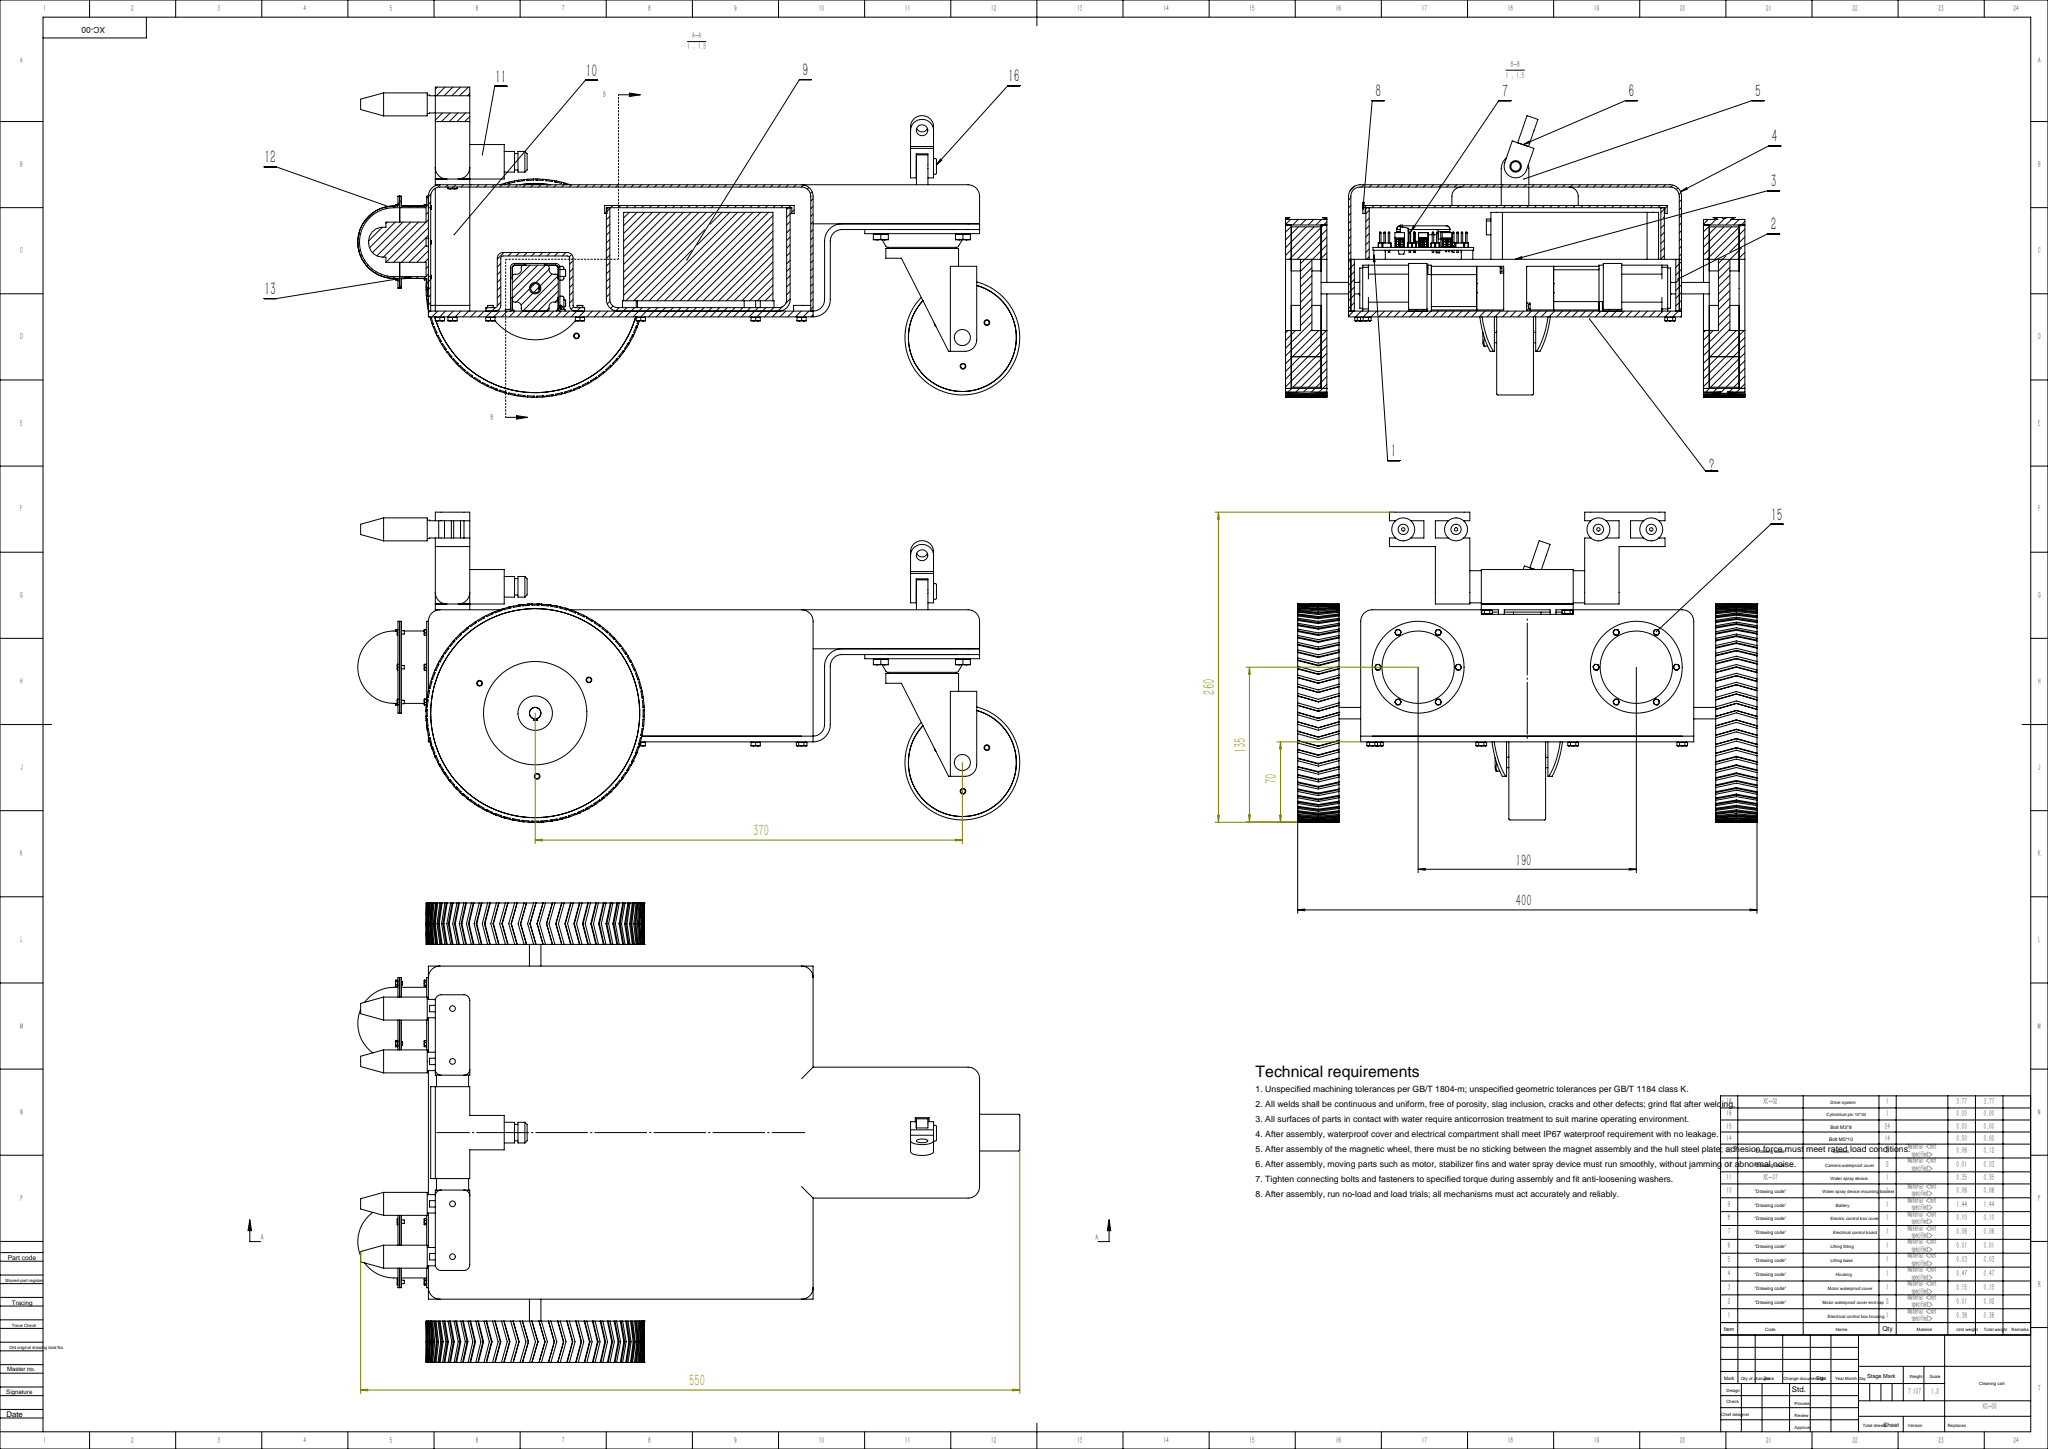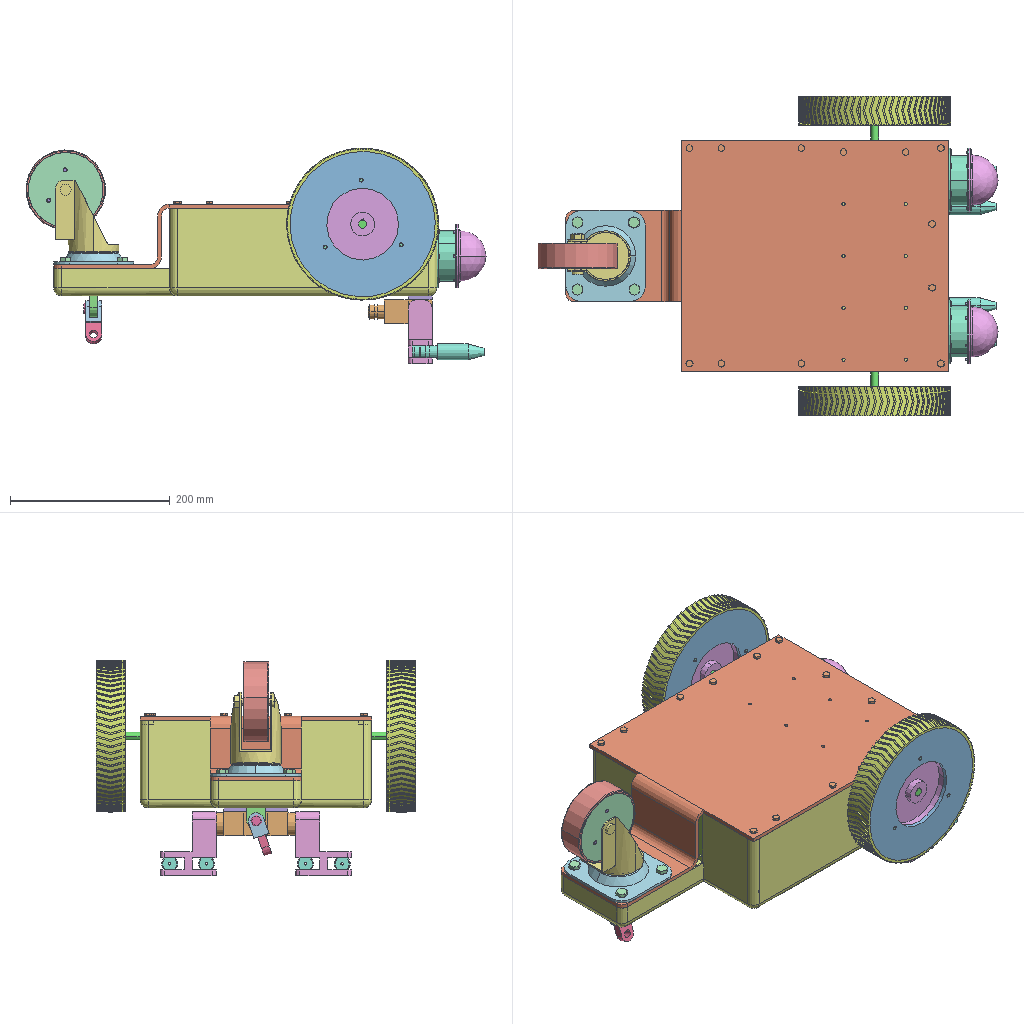Assembly | SolidWorks | 42 different items | 115 placed | box 576 x 400 x 270 mm
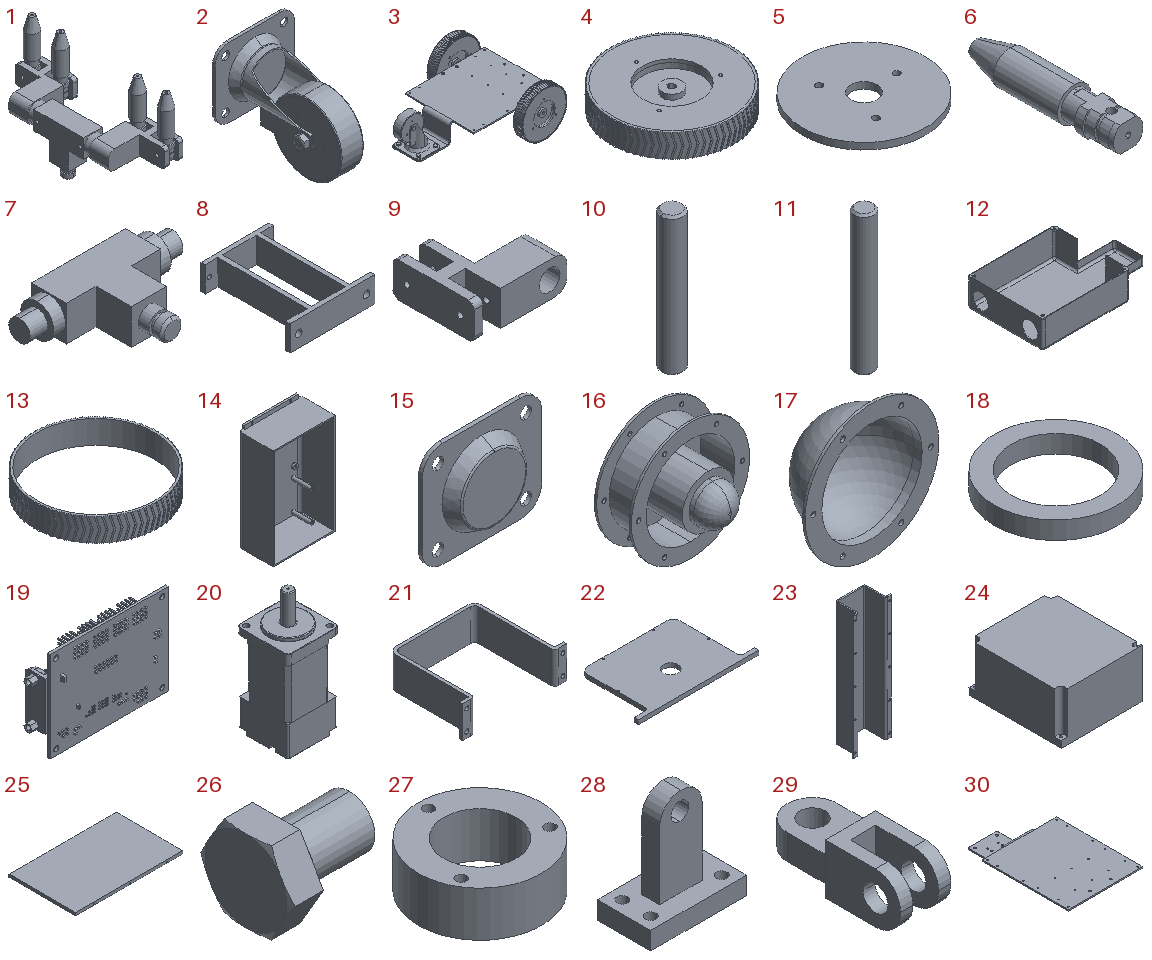Parts list (item | name | quantity | parent item | size | volume | features):
1 | (subassembly) | x1 | - | 80 x 240 x 145 mm | 354979 mm3 | -
2 | (subassembly) | x1 | in 3 | 114 x 144 x 135 mm | 347724 mm3 | features CompositeCurve 1
3 | (subassembly) | x1 | - | 517.127 x 400 x 190.253 mm | 2987569 mm3 | features CompositeCurve 2, LocalLPattern 1
4 | (subassembly) | x2 | in 3 | 190.182 x 190.182 x 36 mm | 833820 mm3 | -
5 | - | x2 | in 2 | 94 x 94 x 5 mm | 32834 mm3 | features Extrusion 1
6 | - | x4 | in 1 | 20 x 90 x 20 mm | 21802 mm3 | features ICE 3, Revolution 1
7 | - | x1 | in 1 | 130 x 80 x 30 mm | 123416 mm3 | features ICE 6, Chamfer 1, Cut 1, Extrusion 1
8 | - | x1 | - | 100 x 115 x 30 mm | 57801 mm3 | features ICE 2, Extrusion 1
9 | - | x2 | in 1 | 80 x 70 x 30 mm | 72177 mm3 | features ICE 3, Fillet 2, Extrusion 1
10 | - | x3 | in 2 | 5 x 5 x 32 mm | 624.653 mm3 | features Chamfer 1, Extrusion 1
11 | - | x6 | in 4 | 5 x 5 x 36 mm | 703.193 mm3 | features Chamfer 1, Extrusion 1
12 | - | x1 | - | 480 x 290 x 110 mm | 467348 mm3 | features ICE 6, Fillet 3, CirPattern 2, Extrusion 1, Shell 1
13 | - | x2 | in 4 | 190.182 x 190.182 x 36 mm | 68309 mm3 | features CirPattern 1, Extrusion 1, ICE 1
14 | - | x1 | - | 160 x 90 x 280 mm | 364305 mm3 | features ICE 5, Extrusion 1, Fillet 1, Shell 1
15 | - | x1 | in 2 | 114 x 15.475 x 100 mm | 79826 mm3 | features RefAxis 6, 3DProfileFeature 2, ICE 2, Extrusion 1, Revolution 1
16 | - | x2 | - | 80 x 52 x 80 mm | 58059 mm3 | features ICE 5, Fillet 1, Revolution 1
17 | - | x2 | - | 80 x 36.5 x 80 mm | 13163 mm3 | features ICE 1, Revolution 1
18 | - | x2 | in 4 | 180 x 180 x 26 mm | 316515 mm3 | features Extrusion 1
19 | - | x1 | - | - | 58876 mm3 | features BaseBody 155, Scale 1
20 | - | x2 | in 3 | 40 x 46.5 x 96 mm | 102158 mm3 | features BaseBody 5
21 | - | x2 | in 3 | 52 x 41.5 x 16 mm | 3067 mm3 | features Extrusion 1, ICE 1
22 | - | x2 | - | 86 x 51 x 3 mm | 9982 mm3 | features Extrusion 1
23 | - | x1 | - | 86 x 51 x 280 mm | 147456 mm3 | features Extrusion 1, ICE 1, LPattern 1
24 | - | x1 | - | 130 x 150 x 77 mm | 1439024 mm3 | features ICE 2, Extrusion 1
25 | - | x1 | - | 265 x 165 x 7 mm | 95885 mm3 | features ICE 2, Extrusion 1, LPattern 1
26 | - | x24 | - | 6.1 x 5.543 x 4.8 mm | 68.566 mm3 | features RevCut 3, Boss 1, Chamfer 1, Extrusion 1, Fillet 1, ICE 1, LPattern 1, Scale 1
27 | - | x1 | in 2 | 60 x 60 x 22 mm | 39741 mm3 | features Extrusion 1
28 | - | x1 | - | 54 x 30 x 60 mm | 25666 mm3 | features ICE 2, Extrusion 1, Fillet 1
29 | - | x1 | - | 20 x 55 x 20 mm | 9495 mm3 | features ICE 2, Extrusion 1
30 | - | x1 | in 3 | 290 x 480 x 81 mm | 601902 mm3 | features Cut 5, ICE 4, Fillet 3, Extrusion 1
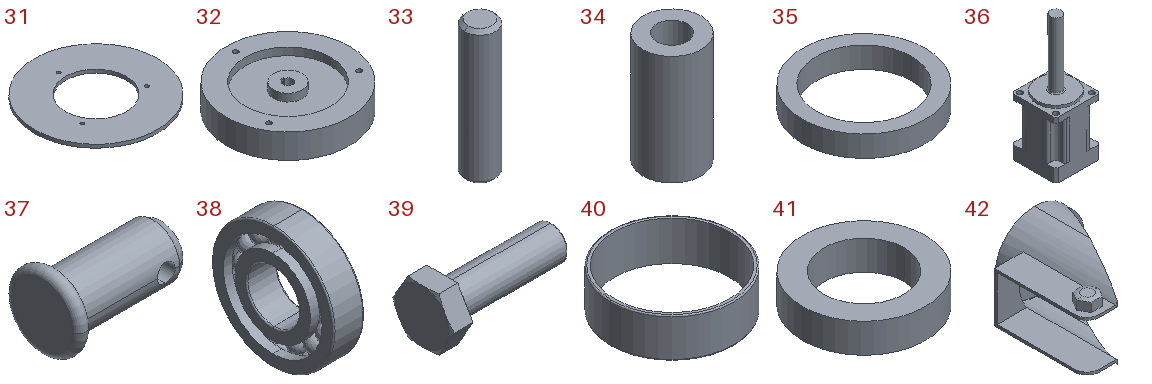31 | - | x4 | in 4 | 182 x 182 x 5 mm | 97974 mm3 | features Extrusion 1
32 | - | x2 | in 4 | 130 x 130 x 26 mm | 250937 mm3 | features ICE 3, Extrusion 1
33 | - | x1 | in 2 | 9 x 9 x 39 mm | 2455 mm3 | features Chamfer 1, Extrusion 1
34 | - | x1 | in 2 | 17 x 17 x 32 mm | 5228 mm3 | features Extrusion 1
35 | - | x1 | in 2 | 35 x 35 x 6 mm | 2337 mm3 | features Extrusion 1
36 | - | x2 | in 3 | 40 x 40 x 114 mm | 76239 mm3 | features ICE 5, BaseBody 1
37 | - | x1 | - | 22.5 x 14 x 14 mm | 1821 mm3 | features Cut 1, Fillet 1, Revolution 1
38 | - | x2 | in 2 | 7 x 28 x 28 mm | 2641 mm3 | features Revolution 3, CirPattern 1, Fillet 1
39 | - | x25 | in 3 | 19.5 x 9.238 x 8 mm | 500.222 mm3 | features RevCut 3, Boss 1, Chamfer 1, Extrusion 1, Fillet 1, LPattern 1
40 | - | x1 | in 2 | 100 x 100 x 32 mm | 29120 mm3 | features Extrusion 1, Fillet 1
41 | - | x1 | in 2 | 92 x 92 x 22 mm | 84044 mm3 | features Extrusion 1
42 | - | x1 | in 2 | 79.167 x 90.525 x 63.333 mm | 28539 mm3 | features RefAxis 15, ICE 6, 3DProfileFeature 5, Revolution 2
Mates (type | each side: item.copy, entity, surface, feature):
In the top assembly
Coincident | 23.1 face plane Boss-Extrude1 | 22.1 face plane Boss-Extrude1 | 3 times
Coincident | 23.1 face plane Boss-Extrude1 | 22.2 face plane Boss-Extrude1
Coincident | 7.1 face plane Boss-Extrude1 | 8.1 face plane Boss-Extrude1 | 3 times
Concentric | 28.1 face cylinder Cut-Extrude1 | 29.1 face cylinder Boss-Extrude2
Coincident | 28.1 face plane Boss-Extrude2 | 29.1 face plane Cut-Extrude1
DistanceDim | 19.1 face plane Input12 | 14.1 face plane Shell1
Concentric | 14.1 face cylinder Boss-Extrude2 | 19.1 face cylinder Input12
Parallel | 14.1 face plane Shell1 | 19.1 face plane Input12
Concentric | 14.1 face cylinder Boss-Extrude3 | 24.1 face cylinder Boss-Extrude1 | 2 times
Coincident | 14.1 face plane Boss-Extrude3 | 24.1 face plane Boss-Extrude1
Coincident | 14.1 face plane Boss-Extrude1 | 25.1 face plane Boss-Extrude1
DistanceDim | 25.1 face plane Boss-Extrude2 | 14.1 face plane Boss-Extrude1 | 2 times
Concentric | 12.1 face cylinder Cut-Extrude5 | 17.1 face cylinder Revolve1
Concentric | 12.1 face cylinder Cut-Extrude5 | 17.2 face cylinder Revolve1
Coincident | 16.1 face plane Revolve1 | 17.2 face plane Revolve1
Concentric | 12.1 face cylinder Cut-Extrude5 | 16.1 face cylinder Revolve1
Concentric | 12.1 face cylinder Cut-Extrude5 | 16.2 face cylinder Revolve1
Concentric | 12.1 face cylinder Cut-Extrude5 | 16.2 face cylinder Cut-Extrude1
Coincident | 12.1 face plane Boss-Extrude1 | 16.2 face plane Revolve1
Coincident | 17.1 face plane Revolve1 | 16.2 face plane Revolve1
Coincident | 17.2 edge | 16.1 face cylinder Cut-Extrude1
Concentric | 17.1 face cylinder Cut-Extrude1 | 16.2 face cylinder Cut-Extrude1
Concentric | 12.1 face cylinder CirPattern2 | 16.1 face cylinder Cut-Extrude1
Concentric | 8.1 face cylinder Cut-Extrude2 | 39.1 face cylinder BaseBody
Coincident | 8.1 face plane Boss-Extrude1 | 39.1 face plane BaseHead
Concentric | 8.1 face cylinder Cut-Extrude2 | 39.2 face cylinder BaseBody
Coincident | 8.1 face plane Boss-Extrude1 | 39.2 face plane BaseHead
Concentric | 14.1 face cylinder Cut-Extrude1 | 39.3 face cylinder BaseBody
Concentric | 16.1 face cylinder Cut-Extrude1 | 26.1 face cylinder BaseBody
Coincident | 17.2 face plane Revolve1 | 26.1 face plane BaseHead
Concentric | 16.1 face cylinder Cut-Extrude1 | 26.2 face cylinder BaseBody
Coincident | 16.1 face plane Revolve1 | 26.2 face plane BaseHead
Concentric | 16.2 face cylinder Cut-Extrude1 | 26.3 face cylinder BaseBody
Coincident | 16.2 face plane Revolve1 | 26.3 face plane BaseHead
Concentric | 16.2 face cylinder Cut-Extrude1 | 26.4 face cylinder BaseBody
Coincident | 16.2 face plane Revolve1 | 26.4 face plane BaseHead
Concentric | 28.1 face cylinder Boss-Extrude1 | 39.4 face cylinder BaseBody
Coincident | 28.1 face plane Boss-Extrude1 | 39.4 face plane BaseHead
Concentric | 28.1 face cylinder Boss-Extrude1 | 39.5 face cylinder BaseBody
Coincident | 28.1 face plane Boss-Extrude1 | 39.5 face plane BaseHead
Concentric | 28.1 face cylinder Boss-Extrude1 | 39.6 face cylinder BaseBody
Coincident | 28.1 face plane Boss-Extrude1 | 39.6 face plane BaseHead
Concentric | 28.1 face cylinder Boss-Extrude1 | 39.7 face cylinder BaseBody
Coincident | 28.1 face plane Boss-Extrude1 | 39.7 face plane BaseHead
Concentric | 29.1 face cylinder Boss-Extrude2 | 37.1 face cylinder BaseBody
Coincident | 29.1 face plane Boss-Extrude2 | 37.1 edge
Coincident | 12.1 face plane Boss-Extrude1 | 30.1 face plane Boss-Extrude1 | 3 times
In subassembly 3
Concentric | 36.1 face cylinder Cut-Extrude2 | 20.1 face cylinder Motor - Copy-1-1-solid1
Coincident | 36.1 face plane Input1 | 20.1 face plane Motor - Copy-1-1-solid2 | 2 times
Concentric | 36.2 face cylinder Cut-Extrude2 | 20.2 face cylinder Motor - Copy-1-1-solid1
Coincident | 36.2 face plane Input1 | 20.2 face plane Motor - Copy-1-1-solid2 | 2 times
Coincident | 20.1 face plane Motor-1-1-solid1 | 20.2 face plane Motor-1-1-solid1
Coincident | 36.1 face plane Input1 | 30.2 face plane Boss-Extrude1
Coincident | 36.1 face plane Input1 | 21.1 face plane Boss-Extrude1 | 3 times
Concentric | 36.1 face cylinder Input1 | 36.2 face cylinder Input1
DistanceDim | 20.1 face plane Motor-1-1-solid1 | 20.2 face plane Motor-1-1-solid1
Coincident | 36.1 face plane Boss-Extrude1 | 32.1 face plane Boss-Extrude1
Coincident | 36.2 face plane Boss-Extrude1 | 32.2 face plane Boss-Extrude1
Coincident | 36.2 face plane Input1 | 21.2 face plane Boss-Extrude1 | 2 times
Coincident | 21.1 face plane Boss-Extrude1 | 21.2 face plane Boss-Extrude1
Concentric | 36.1 face cylinder Input1 | 32.1 face cylinder Cut-Extrude1
Concentric | 36.2 face cylinder Input1 | 31.1 edge
Coincident | 15.1 face plane Boss-Extrude1 | 30.2 face plane Boss-Extrude3 | 2 times
Coincident | 15.1 face plane Boss-Extrude1 | 30.2 face plane Boss-Extrude2
Concentric | 30.2 face cylinder Cut-Extrude6 | 39.8 face cylinder BaseBody
Coincident | 30.2 face plane Boss-Extrude1 | 39.8 face plane BaseHead
Concentric | 15.1 face cylinder Cut-Extrude2 | 39.9 face cylinder BaseBody
Coincident | 15.1 face plane Boss-Extrude1 | 39.9 face plane BaseHead
Concentric | 15.1 face cylinder Cut-Extrude2 | 39.10 face cylinder BaseBody
Coincident | 15.1 face plane Boss-Extrude1 | 39.10 face plane BaseHead
Concentric | 30.2 face cylinder Cut-Extrude2 | 39.11 face cylinder BaseBody
Coincident | 15.1 face plane Boss-Extrude1 | 39.11 face plane BaseHead
Concentric | 30.2 face cylinder Cut-Extrude7 | 39.12 face cylinder BaseBody
Coincident | 30.2 face plane Boss-Extrude1 | 39.12 face plane BaseHead
Concentric | 30.2 face cylinder Cut-Extrude3 | 39.13 face cylinder BaseBody
Coincident | 30.2 face plane Boss-Extrude1 | 39.13 face plane BaseHead
Coincident | 30.2 edge | 39.14 face cylinder BaseBody
Coincident | 15.1 face plane Boss-Extrude1 | 39.14 face plane BaseHead
In subassembly 4
Concentric | 18.1 face cylinder Boss-Extrude1 | 31.2 face cylinder Boss-Extrude1
Coincident | 18.1 face plane Boss-Extrude1 | 31.2 face plane Boss-Extrude1
Concentric | 18.1 face cylinder Boss-Extrude1 | 31.3 face cylinder Boss-Extrude1
Coincident | 18.1 face plane Boss-Extrude1 | 31.3 face plane Boss-Extrude1
Concentric | 31.2 face cylinder Boss-Extrude1 | 13.1 face cylinder Boss-Extrude1
Coincident | 31.2 face plane Boss-Extrude1 | 13.1 face plane Boss-Extrude1
Concentric | 31.2 face cylinder Boss-Extrude1 | 32.3 face cylinder Boss-Extrude1 | 2 times
Coincident | 18.1 face plane Boss-Extrude1 | 32.3 face plane Boss-Extrude1
Concentric | 31.3 face cylinder Boss-Extrude1 | 32.3 face cylinder Boss-Extrude1
Parallel | 32.3 face plane Cut-Extrude1 | 4.1 plane
Concentric | 31.3 face cylinder Boss-Extrude1 | 11.1 face cylinder Boss-Extrude1
Coincident | 31.3 face plane Boss-Extrude1 | 11.1 face plane Boss-Extrude1
Concentric | 31.3 face cylinder Boss-Extrude1 | 11.2 face cylinder Boss-Extrude1
Coincident | 31.3 face plane Boss-Extrude1 | 11.2 face plane Boss-Extrude1
Concentric | 31.3 face cylinder Boss-Extrude1 | 11.3 face cylinder Boss-Extrude1
Coincident | 31.3 face plane Boss-Extrude1 | 11.3 face plane Boss-Extrude1
In subassembly 2
Coincident | 15.2 plane | 42.1 plane
Coincident | 15.2 axis | 42.1 axis
Concentric | 42.1 face cylinder Boss-Extrude2 | 41.1 face cylinder Boss-Extrude1
Concentric | 41.1 face cylinder Boss-Extrude1 | 5.1 face cylinder Boss-Extrude1
Concentric | 41.1 face cylinder Boss-Extrude1 | 5.2 face cylinder Boss-Extrude1
Coincident | 41.1 face plane Boss-Extrude1 | 5.2 face plane Boss-Extrude1
Coincident | 41.1 face plane Boss-Extrude1 | 5.1 face plane Boss-Extrude1
DistanceDim | 5.2 face plane Boss-Extrude1 | 42.1 face plane Cut-Extrude1
Concentric | 5.1 face cylinder Boss-Extrude1 | 40.1 face cylinder Boss-Extrude1
Coincident | 5.1 face plane Boss-Extrude1 | 40.1 face plane Boss-Extrude1
Concentric | 41.1 face cylinder Boss-Extrude1 | 27.1 face cylinder Boss-Extrude1
Coincident | 5.1 face plane Boss-Extrude1 | 27.1 face plane Boss-Extrude1
Concentric | 5.1 face cylinder Boss-Extrude1 | 27.1 face cylinder Boss-Extrude1
Concentric | 27.1 face cylinder Boss-Extrude1 | 38.1 face cylinder Revolve3
Coincident | 27.1 face plane Boss-Extrude1 | 38.1 face plane Revolve3
Concentric | 27.1 face cylinder Boss-Extrude1 | 38.2 face cylinder Revolve3
Coincident | 27.1 face plane Boss-Extrude1 | 38.2 face plane Revolve3
Concentric | 38.1 face cylinder Revolve2 | 35.1 face cylinder Boss-Extrude1
Coincident | 38.1 face plane Revolve3 | 35.1 face plane Boss-Extrude1
Concentric | 38.1 face cylinder Revolve2 | 34.1 face cylinder Boss-Extrude1
Coincident | 40.1 face plane Boss-Extrude1 | 34.1 face plane Boss-Extrude1
Concentric | 34.1 face cylinder Boss-Extrude1 | 33.1 face cylinder Boss-Extrude1
Coincident | 42.1 face plane Boss-Extrude1 | 33.1 face plane Boss-Extrude1
Parallel | 15.2 face plane Boss-Extrude1 | 5.2 face plane Boss-Extrude1
Concentric | 5.2 face cylinder Boss-Extrude1 | 27.1 face cylinder Boss-Extrude1
Concentric | 5.2 face cylinder Boss-Extrude1 | 10.1 face cylinder Boss-Extrude1
Coincident | 5.2 face plane Boss-Extrude1 | 10.1 face plane Boss-Extrude1
Coincident | 5.2 edge | 10.2 face cylinder Boss-Extrude1
Coincident | 5.2 face plane Boss-Extrude1 | 10.2 face plane Boss-Extrude1
Concentric | 5.2 face cylinder Boss-Extrude1 | 10.3 face cylinder Boss-Extrude1
Coincident | 5.2 face plane Boss-Extrude1 | 10.3 face plane Boss-Extrude1
In subassembly 1
Coincident | 9.1 face plane Cut-Extrude3 | 6.1 face plane Cut-Extrude1
Concentric | 9.1 face cylinder Cut-Extrude4 | 6.1 face cylinder Cut-Extrude2
Concentric | 9.1 face cylinder Cut-Extrude4 | 6.2 face cylinder Cut-Extrude2
Coincident | 9.1 face plane Cut-Extrude3 | 6.2 face plane Cut-Extrude1
Concentric | 9.1 face cylinder Cut-Extrude2 | 7.2 face cylinder Boss-Extrude3
Coincident | 9.1 face plane Boss-Extrude1 | 7.2 face plane Boss-Extrude2
Concentric | 7.2 face cylinder Boss-Extrude5 | 9.2 face cylinder Cut-Extrude2
Coincident | 7.2 face plane Boss-Extrude4 | 9.2 face plane Boss-Extrude1
Concentric | 9.2 face cylinder Cut-Extrude4 | 6.3 face cylinder Cut-Extrude2
Coincident | 9.2 face plane Cut-Extrude3 | 6.3 face plane Cut-Extrude1
Concentric | 9.2 face cylinder Cut-Extrude4 | 6.4 face cylinder Cut-Extrude2
Coincident | 9.2 face plane Cut-Extrude3 | 6.4 face plane Cut-Extrude1
Coincident | 9.1 face plane Boss-Extrude1 | 9.2 face plane Boss-Extrude1
Parallel | 7.2 face plane Boss-Extrude1 | 9.2 face plane Boss-Extrude1
Coincident | 7.2 face plane Boss-Extrude1 | 1.1 plane
Parallel | 9.2 face plane Boss-Extrude1 | 6.3 face plane Cut-Extrude1
Parallel | 9.2 face plane Boss-Extrude1 | 6.4 face plane Cut-Extrude1
Parallel | 9.1 face plane Boss-Extrude1 | 6.2 face plane Cut-Extrude1
Parallel | 9.1 face plane Boss-Extrude1 | 6.1 face plane Cut-Extrude1